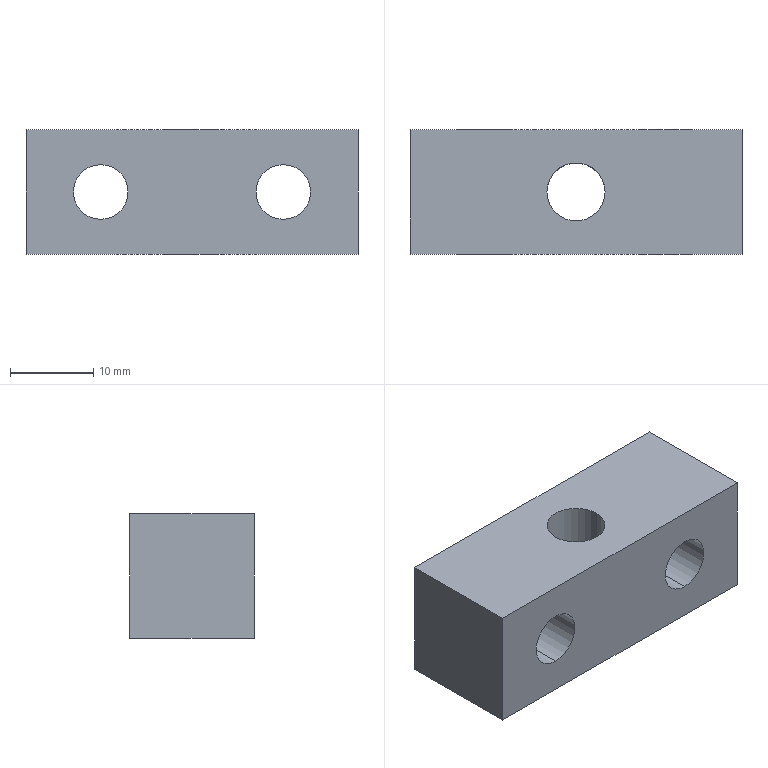Part | STEP file | 0243_212_Block | 1 solid | 12 faces | box 40 x 15 x 15 mm | volume 7396 mm3 | cylinder 6 | plane 6 | commonest cylinder face diameters 6.6 x4 7 x2
STEP:
#1=CARTESIAN_POINT('',(0.,0.,0.));
#2=DIRECTION('',(0.,0.,1.));
#3=DIRECTION('',(1.,0.,0.));
#4=AXIS2_PLACEMENT_3D('',#1,#2,#3);
#5=CARTESIAN_POINT('',(11.,0.,10.8));
#6=VERTEX_POINT('',#5);
#7=CARTESIAN_POINT('',(11.,15.,10.8));
#8=VERTEX_POINT('',#7);
#9=CARTESIAN_POINT('',(11.,15.,10.8));
#10=DIRECTION('',(0.,1.,0.));
#11=VECTOR('',#10,1.);
#12=LINE('',#9,#11);
#13=CARTESIAN_POINT('',(11.,15.,7.5));
#14=DIRECTION('',(0.,1.,0.));
#15=DIRECTION('',(0.,0.,1.));
#16=AXIS2_PLACEMENT_3D('',#13,#14,#15);
#17=CYLINDRICAL_SURFACE('',#16,3.3);
#18=CARTESIAN_POINT('',(6.283,0.));
#19=DIRECTION('',(0.,1.));
#20=VECTOR('',#19,1.);
#21=LINE('',#18,#20);
#22=(GEOMETRIC_REPRESENTATION_CONTEXT(2)PARAMETRIC_REPRESENTATION_CONTEXT()REPRESENTATION_CONTEXT('',''));
#23=DEFINITIONAL_REPRESENTATION('',(#21),#22);
#24=PCURVE('',#17,#23);
#25=CARTESIAN_POINT('',(11.,15.,7.5));
#26=DIRECTION('',(0.,1.,0.));
#27=DIRECTION('',(0.,0.,1.));
#28=AXIS2_PLACEMENT_3D('',#25,#26,#27);
#29=CYLINDRICAL_SURFACE('',#28,3.3);
#30=CARTESIAN_POINT('',(0.,0.));
#31=DIRECTION('',(0.,1.));
#32=VECTOR('',#31,1.);
#33=LINE('',#30,#32);
#34=(GEOMETRIC_REPRESENTATION_CONTEXT(2)PARAMETRIC_REPRESENTATION_CONTEXT()REPRESENTATION_CONTEXT('',''));
#35=DEFINITIONAL_REPRESENTATION('',(#33),#34);
#36=PCURVE('',#29,#35);
#37=SURFACE_CURVE('',#12,(#24,#36),.PCURVE_S1.);
#38=EDGE_CURVE('',#6,#8,#37,.T.);
#39=ORIENTED_EDGE('',*,*,#38,.T.);
#40=CARTESIAN_POINT('',(11.,15.,4.2));
#41=VERTEX_POINT('',#40);
#42=CARTESIAN_POINT('',(11.,15.,7.5));
#43=DIRECTION('',(0.,1.,0.));
#44=DIRECTION('',(0.,0.,1.));
#45=AXIS2_PLACEMENT_3D('',#42,#43,#44);
#46=CIRCLE('',#45,3.3);
#47=CARTESIAN_POINT('',(0.,0.));
#48=DIRECTION('',(1.,0.));
#49=VECTOR('',#48,1.);
#50=LINE('',#47,#49);
#51=(GEOMETRIC_REPRESENTATION_CONTEXT(2)PARAMETRIC_REPRESENTATION_CONTEXT()REPRESENTATION_CONTEXT('',''));
#52=DEFINITIONAL_REPRESENTATION('',(#50),#51);
#53=PCURVE('',#17,#52);
#54=CARTESIAN_POINT('',(-20.,15.,15.));
#55=DIRECTION('',(0.,-1.,0.));
#56=DIRECTION('',(0.,0.,-1.));
#57=AXIS2_PLACEMENT_3D('',#54,#55,#56);
#58=PLANE('',#57);
#59=CARTESIAN_POINT('',(4.2,31.));
#60=CARTESIAN_POINT('',(4.2,36.716));
#61=CARTESIAN_POINT('',(9.15,33.858));
#62=CARTESIAN_POINT('',(14.1,31.));
#63=CARTESIAN_POINT('',(9.15,28.142));
#64=CARTESIAN_POINT('',(4.2,25.284));
#65=CARTESIAN_POINT('',(4.2,31.));
#66=(BOUNDED_CURVE()B_SPLINE_CURVE(2,(#59,#60,#61,#62,#63,#64,#65),.UNSPECIFIED.,.T.,.F.)B_SPLINE_CURVE_WITH_KNOTS((1,2,2,2,2,1),(-2.094,0.,2.094,4.189,6.283,8.378),.UNSPECIFIED.)CURVE()GEOMETRIC_REPRESENTATION_ITEM()RATIONAL_B_SPLINE_CURVE((1.,0.5,1.,0.5,1.,0.5,1.))REPRESENTATION_ITEM(''));
#67=(GEOMETRIC_REPRESENTATION_CONTEXT(2)PARAMETRIC_REPRESENTATION_CONTEXT()REPRESENTATION_CONTEXT('',''));
#68=DEFINITIONAL_REPRESENTATION('',(#66),#67);
#69=PCURVE('',#58,#68);
#70=SURFACE_CURVE('',#46,(#53,#69),.PCURVE_S1.);
#71=EDGE_CURVE('',#41,#8,#70,.T.);
#72=ORIENTED_EDGE('',*,*,#71,.F.);
#73=CARTESIAN_POINT('',(11.,0.,4.2));
#74=VERTEX_POINT('',#73);
#75=CARTESIAN_POINT('',(11.,15.,4.2));
#76=DIRECTION('',(0.,1.,0.));
#77=VECTOR('',#76,1.);
#78=LINE('',#75,#77);
#79=CARTESIAN_POINT('',(3.142,0.));
#80=DIRECTION('',(0.,1.));
#81=VECTOR('',#80,1.);
#82=LINE('',#79,#81);
#83=(GEOMETRIC_REPRESENTATION_CONTEXT(2)PARAMETRIC_REPRESENTATION_CONTEXT()REPRESENTATION_CONTEXT('',''));
#84=DEFINITIONAL_REPRESENTATION('',(#82),#83);
#85=PCURVE('',#17,#84);
#86=CARTESIAN_POINT('',(3.142,0.));
#87=DIRECTION('',(0.,1.));
#88=VECTOR('',#87,1.);
#89=LINE('',#86,#88);
#90=(GEOMETRIC_REPRESENTATION_CONTEXT(2)PARAMETRIC_REPRESENTATION_CONTEXT()REPRESENTATION_CONTEXT('',''));
#91=DEFINITIONAL_REPRESENTATION('',(#89),#90);
#92=PCURVE('',#29,#91);
#93=SURFACE_CURVE('',#78,(#85,#92),.PCURVE_S1.);
#94=EDGE_CURVE('',#74,#41,#93,.T.);
#95=ORIENTED_EDGE('',*,*,#94,.F.);
#96=CARTESIAN_POINT('',(11.,0.,7.5));
#97=DIRECTION('',(0.,1.,0.));
#98=DIRECTION('',(0.,0.,1.));
#99=AXIS2_PLACEMENT_3D('',#96,#97,#98);
#100=CIRCLE('',#99,3.3);
#101=CARTESIAN_POINT('',(0.,-15.));
#102=DIRECTION('',(1.,0.));
#103=VECTOR('',#102,1.);
#104=LINE('',#101,#103);
#105=(GEOMETRIC_REPRESENTATION_CONTEXT(2)PARAMETRIC_REPRESENTATION_CONTEXT()REPRESENTATION_CONTEXT('',''));
#106=DEFINITIONAL_REPRESENTATION('',(#104),#105);
#107=PCURVE('',#17,#106);
#108=CARTESIAN_POINT('',(-20.,0.,15.));
#109=DIRECTION('',(0.,1.,0.));
#110=DIRECTION('',(0.,0.,1.));
#111=AXIS2_PLACEMENT_3D('',#108,#109,#110);
#112=PLANE('',#111);
#113=CARTESIAN_POINT('',(-7.5,31.));
#114=DIRECTION('',(1.,0.));
#115=AXIS2_PLACEMENT_2D('',#113,#114);
#116=CIRCLE('',#115,3.3);
#117=(GEOMETRIC_REPRESENTATION_CONTEXT(2)PARAMETRIC_REPRESENTATION_CONTEXT()REPRESENTATION_CONTEXT('',''));
#118=DEFINITIONAL_REPRESENTATION('',(#116),#117);
#119=PCURVE('',#112,#118);
#120=SURFACE_CURVE('',#100,(#107,#119),.PCURVE_S1.);
#121=EDGE_CURVE('',#74,#6,#120,.T.);
#122=ORIENTED_EDGE('',*,*,#121,.T.);
#123=EDGE_LOOP('',(#39,#72,#95,#122));
#124=FACE_BOUND('',#123,.F.);
#125=ADVANCED_FACE('',(#124),#17,.F.);
#126=CARTESIAN_POINT('',(-11.,0.,10.8));
#127=VERTEX_POINT('',#126);
#128=CARTESIAN_POINT('',(-11.,15.,10.8));
#129=VERTEX_POINT('',#128);
#130=CARTESIAN_POINT('',(-11.,15.,10.8));
#131=DIRECTION('',(0.,1.,0.));
#132=VECTOR('',#131,1.);
#133=LINE('',#130,#132);
#134=CARTESIAN_POINT('',(-11.,15.,7.5));
#135=DIRECTION('',(0.,1.,0.));
#136=DIRECTION('',(0.,0.,1.));
#137=AXIS2_PLACEMENT_3D('',#134,#135,#136);
#138=CYLINDRICAL_SURFACE('',#137,3.3);
#139=CARTESIAN_POINT('',(6.283,0.));
#140=DIRECTION('',(0.,1.));
#141=VECTOR('',#140,1.);
#142=LINE('',#139,#141);
#143=(GEOMETRIC_REPRESENTATION_CONTEXT(2)PARAMETRIC_REPRESENTATION_CONTEXT()REPRESENTATION_CONTEXT('',''));
#144=DEFINITIONAL_REPRESENTATION('',(#142),#143);
#145=PCURVE('',#138,#144);
#146=CARTESIAN_POINT('',(-11.,15.,7.5));
#147=DIRECTION('',(0.,1.,0.));
#148=DIRECTION('',(0.,0.,1.));
#149=AXIS2_PLACEMENT_3D('',#146,#147,#148);
#150=CYLINDRICAL_SURFACE('',#149,3.3);
#151=CARTESIAN_POINT('',(0.,0.));
#152=DIRECTION('',(0.,1.));
#153=VECTOR('',#152,1.);
#154=LINE('',#151,#153);
#155=(GEOMETRIC_REPRESENTATION_CONTEXT(2)PARAMETRIC_REPRESENTATION_CONTEXT()REPRESENTATION_CONTEXT('',''));
#156=DEFINITIONAL_REPRESENTATION('',(#154),#155);
#157=PCURVE('',#150,#156);
#158=SURFACE_CURVE('',#133,(#145,#157),.PCURVE_S1.);
#159=EDGE_CURVE('',#127,#129,#158,.T.);
#160=ORIENTED_EDGE('',*,*,#159,.T.);
#161=CARTESIAN_POINT('',(-11.,15.,4.2));
#162=VERTEX_POINT('',#161);
#163=CARTESIAN_POINT('',(-11.,15.,7.5));
#164=DIRECTION('',(0.,1.,0.));
#165=DIRECTION('',(0.,0.,1.));
#166=AXIS2_PLACEMENT_3D('',#163,#164,#165);
#167=CIRCLE('',#166,3.3);
#168=CARTESIAN_POINT('',(0.,0.));
#169=DIRECTION('',(1.,0.));
#170=VECTOR('',#169,1.);
#171=LINE('',#168,#170);
#172=(GEOMETRIC_REPRESENTATION_CONTEXT(2)PARAMETRIC_REPRESENTATION_CONTEXT()REPRESENTATION_CONTEXT('',''));
#173=DEFINITIONAL_REPRESENTATION('',(#171),#172);
#174=PCURVE('',#138,#173);
#175=CARTESIAN_POINT('',(4.2,9.));
#176=CARTESIAN_POINT('',(4.2,14.716));
#177=CARTESIAN_POINT('',(9.15,11.858));
#178=CARTESIAN_POINT('',(14.1,9.));
#179=CARTESIAN_POINT('',(9.15,6.142));
#180=CARTESIAN_POINT('',(4.2,3.284));
#181=CARTESIAN_POINT('',(4.2,9.));
#182=(BOUNDED_CURVE()B_SPLINE_CURVE(2,(#175,#176,#177,#178,#179,#180,#181),.UNSPECIFIED.,.T.,.F.)B_SPLINE_CURVE_WITH_KNOTS((1,2,2,2,2,1),(-2.094,0.,2.094,4.189,6.283,8.378),.UNSPECIFIED.)CURVE()GEOMETRIC_REPRESENTATION_ITEM()RATIONAL_B_SPLINE_CURVE((1.,0.5,1.,0.5,1.,0.5,1.))REPRESENTATION_ITEM(''));
#183=(GEOMETRIC_REPRESENTATION_CONTEXT(2)PARAMETRIC_REPRESENTATION_CONTEXT()REPRESENTATION_CONTEXT('',''));
#184=DEFINITIONAL_REPRESENTATION('',(#182),#183);
#185=PCURVE('',#58,#184);
#186=SURFACE_CURVE('',#167,(#174,#185),.PCURVE_S1.);
#187=EDGE_CURVE('',#162,#129,#186,.T.);
#188=ORIENTED_EDGE('',*,*,#187,.F.);
#189=CARTESIAN_POINT('',(-11.,0.,4.2));
#190=VERTEX_POINT('',#189);
#191=CARTESIAN_POINT('',(-11.,15.,4.2));
#192=DIRECTION('',(0.,1.,0.));
#193=VECTOR('',#192,1.);
#194=LINE('',#191,#193);
#195=CARTESIAN_POINT('',(3.142,0.));
#196=DIRECTION('',(0.,1.));
#197=VECTOR('',#196,1.);
#198=LINE('',#195,#197);
#199=(GEOMETRIC_REPRESENTATION_CONTEXT(2)PARAMETRIC_REPRESENTATION_CONTEXT()REPRESENTATION_CONTEXT('',''));
#200=DEFINITIONAL_REPRESENTATION('',(#198),#199);
#201=PCURVE('',#138,#200);
#202=CARTESIAN_POINT('',(3.142,0.));
#203=DIRECTION('',(0.,1.));
#204=VECTOR('',#203,1.);
#205=LINE('',#202,#204);
#206=(GEOMETRIC_REPRESENTATION_CONTEXT(2)PARAMETRIC_REPRESENTATION_CONTEXT()REPRESENTATION_CONTEXT('',''));
#207=DEFINITIONAL_REPRESENTATION('',(#205),#206);
#208=PCURVE('',#150,#207);
#209=SURFACE_CURVE('',#194,(#201,#208),.PCURVE_S1.);
#210=EDGE_CURVE('',#190,#162,#209,.T.);
#211=ORIENTED_EDGE('',*,*,#210,.F.);
#212=CARTESIAN_POINT('',(-11.,0.,7.5));
#213=DIRECTION('',(0.,1.,0.));
#214=DIRECTION('',(0.,0.,1.));
#215=AXIS2_PLACEMENT_3D('',#212,#213,#214);
#216=CIRCLE('',#215,3.3);
#217=CARTESIAN_POINT('',(0.,-15.));
#218=DIRECTION('',(1.,0.));
#219=VECTOR('',#218,1.);
#220=LINE('',#217,#219);
#221=(GEOMETRIC_REPRESENTATION_CONTEXT(2)PARAMETRIC_REPRESENTATION_CONTEXT()REPRESENTATION_CONTEXT('',''));
#222=DEFINITIONAL_REPRESENTATION('',(#220),#221);
#223=PCURVE('',#138,#222);
#224=CARTESIAN_POINT('',(-7.5,9.));
#225=DIRECTION('',(1.,0.));
#226=AXIS2_PLACEMENT_2D('',#224,#225);
#227=CIRCLE('',#226,3.3);
#228=(GEOMETRIC_REPRESENTATION_CONTEXT(2)PARAMETRIC_REPRESENTATION_CONTEXT()REPRESENTATION_CONTEXT('',''));
#229=DEFINITIONAL_REPRESENTATION('',(#227),#228);
#230=PCURVE('',#112,#229);
#231=SURFACE_CURVE('',#216,(#223,#230),.PCURVE_S1.);
#232=EDGE_CURVE('',#190,#127,#231,.T.);
#233=ORIENTED_EDGE('',*,*,#232,.T.);
#234=EDGE_LOOP('',(#160,#188,#211,#233));
#235=FACE_BOUND('',#234,.F.);
#236=ADVANCED_FACE('',(#235),#138,.F.);
#237=CARTESIAN_POINT('',(3.5,7.5,0.));
#238=VERTEX_POINT('',#237);
#239=CARTESIAN_POINT('',(3.5,7.5,15.));
#240=VERTEX_POINT('',#239);
#241=CARTESIAN_POINT('',(3.5,7.5,15.));
#242=DIRECTION('',(0.,0.,1.));
#243=VECTOR('',#242,1.);
#244=LINE('',#241,#243);
#245=CARTESIAN_POINT('',(0.,7.5,15.));
#246=DIRECTION('',(0.,0.,1.));
#247=DIRECTION('',(1.,0.,0.));
#248=AXIS2_PLACEMENT_3D('',#245,#246,#247);
#249=CYLINDRICAL_SURFACE('',#248,3.5);
#250=CARTESIAN_POINT('',(6.283,0.));
#251=DIRECTION('',(0.,1.));
#252=VECTOR('',#251,1.);
#253=LINE('',#250,#252);
#254=(GEOMETRIC_REPRESENTATION_CONTEXT(2)PARAMETRIC_REPRESENTATION_CONTEXT()REPRESENTATION_CONTEXT('',''));
#255=DEFINITIONAL_REPRESENTATION('',(#253),#254);
#256=PCURVE('',#249,#255);
#257=CARTESIAN_POINT('',(0.,7.5,15.));
#258=DIRECTION('',(0.,0.,1.));
#259=DIRECTION('',(1.,0.,0.));
#260=AXIS2_PLACEMENT_3D('',#257,#258,#259);
#261=CYLINDRICAL_SURFACE('',#260,3.5);
#262=CARTESIAN_POINT('',(0.,0.));
#263=DIRECTION('',(0.,1.));
#264=VECTOR('',#263,1.);
#265=LINE('',#262,#264);
#266=(GEOMETRIC_REPRESENTATION_CONTEXT(2)PARAMETRIC_REPRESENTATION_CONTEXT()REPRESENTATION_CONTEXT('',''));
#267=DEFINITIONAL_REPRESENTATION('',(#265),#266);
#268=PCURVE('',#261,#267);
#269=SURFACE_CURVE('',#244,(#256,#268),.PCURVE_S1.);
#270=EDGE_CURVE('',#238,#240,#269,.T.);
#271=ORIENTED_EDGE('',*,*,#270,.T.);
#272=CARTESIAN_POINT('',(-3.5,7.5,15.));
#273=VERTEX_POINT('',#272);
#274=CARTESIAN_POINT('',(0.,7.5,15.));
#275=DIRECTION('',(0.,0.,1.));
#276=DIRECTION('',(1.,0.,0.));
#277=AXIS2_PLACEMENT_3D('',#274,#275,#276);
#278=CIRCLE('',#277,3.5);
#279=CARTESIAN_POINT('',(0.,0.));
#280=DIRECTION('',(1.,0.));
#281=VECTOR('',#280,1.);
#282=LINE('',#279,#281);
#283=(GEOMETRIC_REPRESENTATION_CONTEXT(2)PARAMETRIC_REPRESENTATION_CONTEXT()REPRESENTATION_CONTEXT('',''));
#284=DEFINITIONAL_REPRESENTATION('',(#282),#283);
#285=PCURVE('',#249,#284);
#286=CARTESIAN_POINT('',(-20.,15.,15.));
#287=DIRECTION('',(0.,0.,-1.));
#288=DIRECTION('',(-1.,0.,0.));
#289=AXIS2_PLACEMENT_3D('',#286,#287,#288);
#290=PLANE('',#289);
#291=CARTESIAN_POINT('',(-23.5,-7.5));
#292=CARTESIAN_POINT('',(-23.5,-1.438));
#293=CARTESIAN_POINT('',(-18.25,-4.469));
#294=CARTESIAN_POINT('',(-13.,-7.5));
#295=CARTESIAN_POINT('',(-18.25,-10.531));
#296=CARTESIAN_POINT('',(-23.5,-13.562));
#297=CARTESIAN_POINT('',(-23.5,-7.5));
#298=(BOUNDED_CURVE()B_SPLINE_CURVE(2,(#291,#292,#293,#294,#295,#296,#297),.UNSPECIFIED.,.T.,.F.)B_SPLINE_CURVE_WITH_KNOTS((1,2,2,2,2,1),(-2.094,0.,2.094,4.189,6.283,8.378),.UNSPECIFIED.)CURVE()GEOMETRIC_REPRESENTATION_ITEM()RATIONAL_B_SPLINE_CURVE((1.,0.5,1.,0.5,1.,0.5,1.))REPRESENTATION_ITEM(''));
#299=(GEOMETRIC_REPRESENTATION_CONTEXT(2)PARAMETRIC_REPRESENTATION_CONTEXT()REPRESENTATION_CONTEXT('',''));
#300=DEFINITIONAL_REPRESENTATION('',(#298),#299);
#301=PCURVE('',#290,#300);
#302=SURFACE_CURVE('',#278,(#285,#301),.PCURVE_S1.);
#303=EDGE_CURVE('',#273,#240,#302,.T.);
#304=ORIENTED_EDGE('',*,*,#303,.F.);
#305=CARTESIAN_POINT('',(-3.5,7.5,0.));
#306=VERTEX_POINT('',#305);
#307=CARTESIAN_POINT('',(-3.5,7.5,15.));
#308=DIRECTION('',(0.,0.,1.));
#309=VECTOR('',#308,1.);
#310=LINE('',#307,#309);
#311=CARTESIAN_POINT('',(3.142,0.));
#312=DIRECTION('',(0.,1.));
#313=VECTOR('',#312,1.);
#314=LINE('',#311,#313);
#315=(GEOMETRIC_REPRESENTATION_CONTEXT(2)PARAMETRIC_REPRESENTATION_CONTEXT()REPRESENTATION_CONTEXT('',''));
#316=DEFINITIONAL_REPRESENTATION('',(#314),#315);
#317=PCURVE('',#249,#316);
#318=CARTESIAN_POINT('',(3.142,0.));
#319=DIRECTION('',(0.,1.));
#320=VECTOR('',#319,1.);
#321=LINE('',#318,#320);
#322=(GEOMETRIC_REPRESENTATION_CONTEXT(2)PARAMETRIC_REPRESENTATION_CONTEXT()REPRESENTATION_CONTEXT('',''));
#323=DEFINITIONAL_REPRESENTATION('',(#321),#322);
#324=PCURVE('',#261,#323);
#325=SURFACE_CURVE('',#310,(#317,#324),.PCURVE_S1.);
#326=EDGE_CURVE('',#306,#273,#325,.T.);
#327=ORIENTED_EDGE('',*,*,#326,.F.);
#328=CARTESIAN_POINT('',(0.,7.5,0.));
#329=DIRECTION('',(0.,0.,1.));
#330=DIRECTION('',(1.,0.,0.));
#331=AXIS2_PLACEMENT_3D('',#328,#329,#330);
#332=CIRCLE('',#331,3.5);
#333=CARTESIAN_POINT('',(0.,-15.));
#334=DIRECTION('',(1.,0.));
#335=VECTOR('',#334,1.);
#336=LINE('',#333,#335);
#337=(GEOMETRIC_REPRESENTATION_CONTEXT(2)PARAMETRIC_REPRESENTATION_CONTEXT()REPRESENTATION_CONTEXT('',''));
#338=DEFINITIONAL_REPRESENTATION('',(#336),#337);
#339=PCURVE('',#249,#338);
#340=CARTESIAN_POINT('',(-20.,15.,0.));
#341=DIRECTION('',(0.,0.,-1.));
#342=DIRECTION('',(-1.,0.,0.));
#343=AXIS2_PLACEMENT_3D('',#340,#341,#342);
#344=PLANE('',#343);
#345=CARTESIAN_POINT('',(-23.5,-7.5));
#346=CARTESIAN_POINT('',(-23.5,-1.438));
#347=CARTESIAN_POINT('',(-18.25,-4.469));
#348=CARTESIAN_POINT('',(-13.,-7.5));
#349=CARTESIAN_POINT('',(-18.25,-10.531));
#350=CARTESIAN_POINT('',(-23.5,-13.562));
#351=CARTESIAN_POINT('',(-23.5,-7.5));
#352=(BOUNDED_CURVE()B_SPLINE_CURVE(2,(#345,#346,#347,#348,#349,#350,#351),.UNSPECIFIED.,.T.,.F.)B_SPLINE_CURVE_WITH_KNOTS((1,2,2,2,2,1),(-2.094,0.,2.094,4.189,6.283,8.378),.UNSPECIFIED.)CURVE()GEOMETRIC_REPRESENTATION_ITEM()RATIONAL_B_SPLINE_CURVE((1.,0.5,1.,0.5,1.,0.5,1.))REPRESENTATION_ITEM(''));
#353=(GEOMETRIC_REPRESENTATION_CONTEXT(2)PARAMETRIC_REPRESENTATION_CONTEXT()REPRESENTATION_CONTEXT('',''));
#354=DEFINITIONAL_REPRESENTATION('',(#352),#353);
#355=PCURVE('',#344,#354);
#356=SURFACE_CURVE('',#332,(#339,#355),.PCURVE_S1.);
#357=EDGE_CURVE('',#306,#238,#356,.T.);
#358=ORIENTED_EDGE('',*,*,#357,.T.);
#359=EDGE_LOOP('',(#271,#304,#327,#358));
#360=FACE_BOUND('',#359,.F.);
#361=ADVANCED_FACE('',(#360),#249,.F.);
#362=CARTESIAN_POINT('',(-20.,15.,0.));
#363=VERTEX_POINT('',#362);
#364=CARTESIAN_POINT('',(-20.,0.,0.));
#365=VERTEX_POINT('',#364);
#366=CARTESIAN_POINT('',(-20.,0.,0.));
#367=DIRECTION('',(0.,-1.,0.));
#368=VECTOR('',#367,1.);
#369=LINE('',#366,#368);
#370=CARTESIAN_POINT('',(-20.,0.,15.));
#371=DIRECTION('',(1.,0.,0.));
#372=DIRECTION('',(0.,0.,-1.));
#373=AXIS2_PLACEMENT_3D('',#370,#371,#372);
#374=PLANE('',#373);
#375=CARTESIAN_POINT('',(15.,0.));
#376=DIRECTION('',(0.,-1.));
#377=VECTOR('',#376,1.);
#378=LINE('',#375,#377);
#379=(GEOMETRIC_REPRESENTATION_CONTEXT(2)PARAMETRIC_REPRESENTATION_CONTEXT()REPRESENTATION_CONTEXT('',''));
#380=DEFINITIONAL_REPRESENTATION('',(#378),#379);
#381=PCURVE('',#374,#380);
#382=CARTESIAN_POINT('',(0.,-15.));
#383=DIRECTION('',(0.,-1.));
#384=VECTOR('',#383,1.);
#385=LINE('',#382,#384);
#386=(GEOMETRIC_REPRESENTATION_CONTEXT(2)PARAMETRIC_REPRESENTATION_CONTEXT()REPRESENTATION_CONTEXT('',''));
#387=DEFINITIONAL_REPRESENTATION('',(#385),#386);
#388=PCURVE('',#344,#387);
#389=SURFACE_CURVE('',#369,(#381,#388),.PCURVE_S1.);
#390=EDGE_CURVE('',#363,#365,#389,.T.);
#391=ORIENTED_EDGE('',*,*,#390,.T.);
#392=CARTESIAN_POINT('',(-20.,0.,15.));
#393=VERTEX_POINT('',#392);
#394=CARTESIAN_POINT('',(-20.,0.,15.));
#395=DIRECTION('',(0.,0.,-1.));
#396=VECTOR('',#395,1.);
#397=LINE('',#394,#396);
#398=CARTESIAN_POINT('',(0.,0.));
#399=DIRECTION('',(1.,0.));
#400=VECTOR('',#399,1.);
#401=LINE('',#398,#400);
#402=(GEOMETRIC_REPRESENTATION_CONTEXT(2)PARAMETRIC_REPRESENTATION_CONTEXT()REPRESENTATION_CONTEXT('',''));
#403=DEFINITIONAL_REPRESENTATION('',(#401),#402);
#404=PCURVE('',#374,#403);
#405=CARTESIAN_POINT('',(0.,0.));
#406=DIRECTION('',(-1.,0.));
#407=VECTOR('',#406,1.);
#408=LINE('',#405,#407);
#409=(GEOMETRIC_REPRESENTATION_CONTEXT(2)PARAMETRIC_REPRESENTATION_CONTEXT()REPRESENTATION_CONTEXT('',''));
#410=DEFINITIONAL_REPRESENTATION('',(#408),#409);
#411=PCURVE('',#112,#410);
#412=SURFACE_CURVE('',#397,(#404,#411),.PCURVE_S1.);
#413=EDGE_CURVE('',#393,#365,#412,.T.);
#414=ORIENTED_EDGE('',*,*,#413,.F.);
#415=CARTESIAN_POINT('',(-20.,15.,15.));
#416=VERTEX_POINT('',#415);
#417=CARTESIAN_POINT('',(-20.,0.,15.));
#418=DIRECTION('',(0.,-1.,0.));
#419=VECTOR('',#418,1.);
#420=LINE('',#417,#419);
#421=CARTESIAN_POINT('',(0.,0.));
#422=DIRECTION('',(0.,-1.));
#423=VECTOR('',#422,1.);
#424=LINE('',#421,#423);
#425=(GEOMETRIC_REPRESENTATION_CONTEXT(2)PARAMETRIC_REPRESENTATION_CONTEXT()REPRESENTATION_CONTEXT('',''));
#426=DEFINITIONAL_REPRESENTATION('',(#424),#425);
#427=PCURVE('',#374,#426);
#428=CARTESIAN_POINT('',(0.,-15.));
#429=DIRECTION('',(0.,-1.));
#430=VECTOR('',#429,1.);
#431=LINE('',#428,#430);
#432=(GEOMETRIC_REPRESENTATION_CONTEXT(2)PARAMETRIC_REPRESENTATION_CONTEXT()REPRESENTATION_CONTEXT('',''));
#433=DEFINITIONAL_REPRESENTATION('',(#431),#432);
#434=PCURVE('',#290,#433);
#435=SURFACE_CURVE('',#420,(#427,#434),.PCURVE_S1.);
#436=EDGE_CURVE('',#416,#393,#435,.T.);
#437=ORIENTED_EDGE('',*,*,#436,.F.);
#438=CARTESIAN_POINT('',(-20.,15.,15.));
#439=DIRECTION('',(0.,0.,-1.));
#440=VECTOR('',#439,1.);
#441=LINE('',#438,#440);
#442=CARTESIAN_POINT('',(0.,15.));
#443=DIRECTION('',(1.,0.));
#444=VECTOR('',#443,1.);
#445=LINE('',#442,#444);
#446=(GEOMETRIC_REPRESENTATION_CONTEXT(2)PARAMETRIC_REPRESENTATION_CONTEXT()REPRESENTATION_CONTEXT('',''));
#447=DEFINITIONAL_REPRESENTATION('',(#445),#446);
#448=PCURVE('',#374,#447);
#449=CARTESIAN_POINT('',(0.,0.));
#450=DIRECTION('',(1.,0.));
#451=VECTOR('',#450,1.);
#452=LINE('',#449,#451);
#453=(GEOMETRIC_REPRESENTATION_CONTEXT(2)PARAMETRIC_REPRESENTATION_CONTEXT()REPRESENTATION_CONTEXT('',''));
#454=DEFINITIONAL_REPRESENTATION('',(#452),#453);
#455=PCURVE('',#58,#454);
#456=SURFACE_CURVE('',#441,(#448,#455),.PCURVE_S1.);
#457=EDGE_CURVE('',#416,#363,#456,.T.);
#458=ORIENTED_EDGE('',*,*,#457,.T.);
#459=EDGE_LOOP('',(#391,#414,#437,#458));
#460=FACE_BOUND('',#459,.T.);
#461=ADVANCED_FACE('',(#460),#374,.F.);
#462=CARTESIAN_POINT('',(11.,0.,7.5));
#463=DIRECTION('',(0.,1.,0.));
#464=DIRECTION('',(0.,0.,1.));
#465=AXIS2_PLACEMENT_3D('',#462,#463,#464);
#466=CIRCLE('',#465,3.3);
#467=CARTESIAN_POINT('',(-7.5,31.));
#468=DIRECTION('',(1.,0.));
#469=AXIS2_PLACEMENT_2D('',#467,#468);
#470=CIRCLE('',#469,3.3);
#471=(GEOMETRIC_REPRESENTATION_CONTEXT(2)PARAMETRIC_REPRESENTATION_CONTEXT()REPRESENTATION_CONTEXT('',''));
#472=DEFINITIONAL_REPRESENTATION('',(#470),#471);
#473=PCURVE('',#112,#472);
#474=CARTESIAN_POINT('',(0.,-15.));
#475=DIRECTION('',(1.,0.));
#476=VECTOR('',#475,1.);
#477=LINE('',#474,#476);
#478=(GEOMETRIC_REPRESENTATION_CONTEXT(2)PARAMETRIC_REPRESENTATION_CONTEXT()REPRESENTATION_CONTEXT('',''));
#479=DEFINITIONAL_REPRESENTATION('',(#477),#478);
#480=PCURVE('',#29,#479);
#481=SURFACE_CURVE('',#466,(#473,#480),.PCURVE_S1.);
#482=EDGE_CURVE('',#6,#74,#481,.T.);
#483=ORIENTED_EDGE('',*,*,#482,.T.);
#484=ORIENTED_EDGE('',*,*,#121,.T.);
#485=EDGE_LOOP('',(#483,#484));
#486=FACE_BOUND('',#485,.T.);
#487=CARTESIAN_POINT('',(-11.,0.,7.5));
#488=DIRECTION('',(0.,1.,0.));
#489=DIRECTION('',(0.,0.,1.));
#490=AXIS2_PLACEMENT_3D('',#487,#488,#489);
#491=CIRCLE('',#490,3.3);
#492=CARTESIAN_POINT('',(-7.5,9.));
#493=DIRECTION('',(1.,0.));
#494=AXIS2_PLACEMENT_2D('',#492,#493);
#495=CIRCLE('',#494,3.3);
#496=(GEOMETRIC_REPRESENTATION_CONTEXT(2)PARAMETRIC_REPRESENTATION_CONTEXT()REPRESENTATION_CONTEXT('',''));
#497=DEFINITIONAL_REPRESENTATION('',(#495),#496);
#498=PCURVE('',#112,#497);
#499=CARTESIAN_POINT('',(0.,-15.));
#500=DIRECTION('',(1.,0.));
#501=VECTOR('',#500,1.);
#502=LINE('',#499,#501);
#503=(GEOMETRIC_REPRESENTATION_CONTEXT(2)PARAMETRIC_REPRESENTATION_CONTEXT()REPRESENTATION_CONTEXT('',''));
#504=DEFINITIONAL_REPRESENTATION('',(#502),#503);
#505=PCURVE('',#150,#504);
#506=SURFACE_CURVE('',#491,(#498,#505),.PCURVE_S1.);
#507=EDGE_CURVE('',#127,#190,#506,.T.);
#508=ORIENTED_EDGE('',*,*,#507,.T.);
#509=ORIENTED_EDGE('',*,*,#232,.T.);
#510=EDGE_LOOP('',(#508,#509));
#511=FACE_BOUND('',#510,.T.);
#512=CARTESIAN_POINT('',(20.,0.,0.));
#513=VERTEX_POINT('',#512);
#514=CARTESIAN_POINT('',(-20.,0.,0.));
#515=DIRECTION('',(1.,0.,0.));
#516=VECTOR('',#515,1.);
#517=LINE('',#514,#516);
#518=CARTESIAN_POINT('',(-15.,0.));
#519=DIRECTION('',(0.,1.));
#520=VECTOR('',#519,1.);
#521=LINE('',#518,#520);
#522=(GEOMETRIC_REPRESENTATION_CONTEXT(2)PARAMETRIC_REPRESENTATION_CONTEXT()REPRESENTATION_CONTEXT('',''));
#523=DEFINITIONAL_REPRESENTATION('',(#521),#522);
#524=PCURVE('',#112,#523);
#525=CARTESIAN_POINT('',(0.,-15.));
#526=DIRECTION('',(-1.,0.));
#527=VECTOR('',#526,1.);
#528=LINE('',#525,#527);
#529=(GEOMETRIC_REPRESENTATION_CONTEXT(2)PARAMETRIC_REPRESENTATION_CONTEXT()REPRESENTATION_CONTEXT('',''));
#530=DEFINITIONAL_REPRESENTATION('',(#528),#529);
#531=PCURVE('',#344,#530);
#532=SURFACE_CURVE('',#517,(#524,#531),.PCURVE_S1.);
#533=EDGE_CURVE('',#365,#513,#532,.T.);
#534=ORIENTED_EDGE('',*,*,#533,.T.);
#535=CARTESIAN_POINT('',(20.,0.,15.));
#536=VERTEX_POINT('',#535);
#537=CARTESIAN_POINT('',(20.,0.,15.));
#538=DIRECTION('',(0.,0.,-1.));
#539=VECTOR('',#538,1.);
#540=LINE('',#537,#539);
#541=CARTESIAN_POINT('',(0.,40.));
#542=DIRECTION('',(-1.,0.));
#543=VECTOR('',#542,1.);
#544=LINE('',#541,#543);
#545=(GEOMETRIC_REPRESENTATION_CONTEXT(2)PARAMETRIC_REPRESENTATION_CONTEXT()REPRESENTATION_CONTEXT('',''));
#546=DEFINITIONAL_REPRESENTATION('',(#544),#545);
#547=PCURVE('',#112,#546);
#548=CARTESIAN_POINT('',(20.,0.,15.));
#549=DIRECTION('',(-1.,0.,0.));
#550=DIRECTION('',(0.,0.,1.));
#551=AXIS2_PLACEMENT_3D('',#548,#549,#550);
#552=PLANE('',#551);
#553=CARTESIAN_POINT('',(0.,0.));
#554=DIRECTION('',(-1.,0.));
#555=VECTOR('',#554,1.);
#556=LINE('',#553,#555);
#557=(GEOMETRIC_REPRESENTATION_CONTEXT(2)PARAMETRIC_REPRESENTATION_CONTEXT()REPRESENTATION_CONTEXT('',''));
#558=DEFINITIONAL_REPRESENTATION('',(#556),#557);
#559=PCURVE('',#552,#558);
#560=SURFACE_CURVE('',#540,(#547,#559),.PCURVE_S1.);
#561=EDGE_CURVE('',#536,#513,#560,.T.);
#562=ORIENTED_EDGE('',*,*,#561,.F.);
#563=CARTESIAN_POINT('',(-20.,0.,15.));
#564=DIRECTION('',(1.,0.,0.));
#565=VECTOR('',#564,1.);
#566=LINE('',#563,#565);
#567=CARTESIAN_POINT('',(0.,0.));
#568=DIRECTION('',(0.,1.));
#569=VECTOR('',#568,1.);
#570=LINE('',#567,#569);
#571=(GEOMETRIC_REPRESENTATION_CONTEXT(2)PARAMETRIC_REPRESENTATION_CONTEXT()REPRESENTATION_CONTEXT('',''));
#572=DEFINITIONAL_REPRESENTATION('',(#570),#571);
#573=PCURVE('',#112,#572);
#574=CARTESIAN_POINT('',(0.,-15.));
#575=DIRECTION('',(-1.,0.));
#576=VECTOR('',#575,1.);
#577=LINE('',#574,#576);
#578=(GEOMETRIC_REPRESENTATION_CONTEXT(2)PARAMETRIC_REPRESENTATION_CONTEXT()REPRESENTATION_CONTEXT('',''));
#579=DEFINITIONAL_REPRESENTATION('',(#577),#578);
#580=PCURVE('',#290,#579);
#581=SURFACE_CURVE('',#566,(#573,#580),.PCURVE_S1.);
#582=EDGE_CURVE('',#393,#536,#581,.T.);
#583=ORIENTED_EDGE('',*,*,#582,.F.);
#584=ORIENTED_EDGE('',*,*,#413,.T.);
#585=EDGE_LOOP('',(#534,#562,#583,#584));
#586=FACE_BOUND('',#585,.T.);
#587=ADVANCED_FACE('',(#486,#511,#586),#112,.F.);
#588=CARTESIAN_POINT('',(20.,15.,0.));
#589=VERTEX_POINT('',#588);
#590=CARTESIAN_POINT('',(20.,0.,0.));
#591=DIRECTION('',(0.,1.,0.));
#592=VECTOR('',#591,1.);
#593=LINE('',#590,#592);
#594=CARTESIAN_POINT('',(-15.,0.));
#595=DIRECTION('',(0.,1.));
#596=VECTOR('',#595,1.);
#597=LINE('',#594,#596);
#598=(GEOMETRIC_REPRESENTATION_CONTEXT(2)PARAMETRIC_REPRESENTATION_CONTEXT()REPRESENTATION_CONTEXT('',''));
#599=DEFINITIONAL_REPRESENTATION('',(#597),#598);
#600=PCURVE('',#552,#599);
#601=CARTESIAN_POINT('',(-40.,-15.));
#602=DIRECTION('',(0.,1.));
#603=VECTOR('',#602,1.);
#604=LINE('',#601,#603);
#605=(GEOMETRIC_REPRESENTATION_CONTEXT(2)PARAMETRIC_REPRESENTATION_CONTEXT()REPRESENTATION_CONTEXT('',''));
#606=DEFINITIONAL_REPRESENTATION('',(#604),#605);
#607=PCURVE('',#344,#606);
#608=SURFACE_CURVE('',#593,(#600,#607),.PCURVE_S1.);
#609=EDGE_CURVE('',#513,#589,#608,.T.);
#610=ORIENTED_EDGE('',*,*,#609,.T.);
#611=CARTESIAN_POINT('',(20.,15.,15.));
#612=VERTEX_POINT('',#611);
#613=CARTESIAN_POINT('',(20.,15.,15.));
#614=DIRECTION('',(0.,0.,-1.));
#615=VECTOR('',#614,1.);
#616=LINE('',#613,#615);
#617=CARTESIAN_POINT('',(0.,15.));
#618=DIRECTION('',(-1.,0.));
#619=VECTOR('',#618,1.);
#620=LINE('',#617,#619);
#621=(GEOMETRIC_REPRESENTATION_CONTEXT(2)PARAMETRIC_REPRESENTATION_CONTEXT()REPRESENTATION_CONTEXT('',''));
#622=DEFINITIONAL_REPRESENTATION('',(#620),#621);
#623=PCURVE('',#552,#622);
#624=CARTESIAN_POINT('',(0.,40.));
#625=DIRECTION('',(1.,0.));
#626=VECTOR('',#625,1.);
#627=LINE('',#624,#626);
#628=(GEOMETRIC_REPRESENTATION_CONTEXT(2)PARAMETRIC_REPRESENTATION_CONTEXT()REPRESENTATION_CONTEXT('',''));
#629=DEFINITIONAL_REPRESENTATION('',(#627),#628);
#630=PCURVE('',#58,#629);
#631=SURFACE_CURVE('',#616,(#623,#630),.PCURVE_S1.);
#632=EDGE_CURVE('',#612,#589,#631,.T.);
#633=ORIENTED_EDGE('',*,*,#632,.F.);
#634=CARTESIAN_POINT('',(20.,0.,15.));
#635=DIRECTION('',(0.,1.,0.));
#636=VECTOR('',#635,1.);
#637=LINE('',#634,#636);
#638=CARTESIAN_POINT('',(0.,0.));
#639=DIRECTION('',(0.,1.));
#640=VECTOR('',#639,1.);
#641=LINE('',#638,#640);
#642=(GEOMETRIC_REPRESENTATION_CONTEXT(2)PARAMETRIC_REPRESENTATION_CONTEXT()REPRESENTATION_CONTEXT('',''));
#643=DEFINITIONAL_REPRESENTATION('',(#641),#642);
#644=PCURVE('',#552,#643);
#645=CARTESIAN_POINT('',(-40.,-15.));
#646=DIRECTION('',(0.,1.));
#647=VECTOR('',#646,1.);
#648=LINE('',#645,#647);
#649=(GEOMETRIC_REPRESENTATION_CONTEXT(2)PARAMETRIC_REPRESENTATION_CONTEXT()REPRESENTATION_CONTEXT('',''));
#650=DEFINITIONAL_REPRESENTATION('',(#648),#649);
#651=PCURVE('',#290,#650);
#652=SURFACE_CURVE('',#637,(#644,#651),.PCURVE_S1.);
#653=EDGE_CURVE('',#536,#612,#652,.T.);
#654=ORIENTED_EDGE('',*,*,#653,.F.);
#655=ORIENTED_EDGE('',*,*,#561,.T.);
#656=EDGE_LOOP('',(#610,#633,#654,#655));
#657=FACE_BOUND('',#656,.T.);
#658=ADVANCED_FACE('',(#657),#552,.F.);
#659=CARTESIAN_POINT('',(11.,15.,7.5));
#660=DIRECTION('',(0.,1.,0.));
#661=DIRECTION('',(0.,0.,1.));
#662=AXIS2_PLACEMENT_3D('',#659,#660,#661);
#663=CIRCLE('',#662,3.3);
#664=CARTESIAN_POINT('',(4.2,31.));
#665=CARTESIAN_POINT('',(4.2,36.716));
#666=CARTESIAN_POINT('',(9.15,33.858));
#667=CARTESIAN_POINT('',(14.1,31.));
#668=CARTESIAN_POINT('',(9.15,28.142));
#669=CARTESIAN_POINT('',(4.2,25.284));
#670=CARTESIAN_POINT('',(4.2,31.));
#671=(BOUNDED_CURVE()B_SPLINE_CURVE(2,(#664,#665,#666,#667,#668,#669,#670),.UNSPECIFIED.,.T.,.F.)B_SPLINE_CURVE_WITH_KNOTS((1,2,2,2,2,1),(-2.094,0.,2.094,4.189,6.283,8.378),.UNSPECIFIED.)CURVE()GEOMETRIC_REPRESENTATION_ITEM()RATIONAL_B_SPLINE_CURVE((1.,0.5,1.,0.5,1.,0.5,1.))REPRESENTATION_ITEM(''));
#672=(GEOMETRIC_REPRESENTATION_CONTEXT(2)PARAMETRIC_REPRESENTATION_CONTEXT()REPRESENTATION_CONTEXT('',''));
#673=DEFINITIONAL_REPRESENTATION('',(#671),#672);
#674=PCURVE('',#58,#673);
#675=CARTESIAN_POINT('',(0.,0.));
#676=DIRECTION('',(1.,0.));
#677=VECTOR('',#676,1.);
#678=LINE('',#675,#677);
#679=(GEOMETRIC_REPRESENTATION_CONTEXT(2)PARAMETRIC_REPRESENTATION_CONTEXT()REPRESENTATION_CONTEXT('',''));
#680=DEFINITIONAL_REPRESENTATION('',(#678),#679);
#681=PCURVE('',#29,#680);
#682=SURFACE_CURVE('',#663,(#674,#681),.PCURVE_S1.);
#683=EDGE_CURVE('',#8,#41,#682,.T.);
#684=ORIENTED_EDGE('',*,*,#683,.F.);
#685=ORIENTED_EDGE('',*,*,#71,.F.);
#686=EDGE_LOOP('',(#684,#685));
#687=FACE_BOUND('',#686,.T.);
#688=CARTESIAN_POINT('',(-11.,15.,7.5));
#689=DIRECTION('',(0.,1.,0.));
#690=DIRECTION('',(0.,0.,1.));
#691=AXIS2_PLACEMENT_3D('',#688,#689,#690);
#692=CIRCLE('',#691,3.3);
#693=CARTESIAN_POINT('',(4.2,9.));
#694=CARTESIAN_POINT('',(4.2,14.716));
#695=CARTESIAN_POINT('',(9.15,11.858));
#696=CARTESIAN_POINT('',(14.1,9.));
#697=CARTESIAN_POINT('',(9.15,6.142));
#698=CARTESIAN_POINT('',(4.2,3.284));
#699=CARTESIAN_POINT('',(4.2,9.));
#700=(BOUNDED_CURVE()B_SPLINE_CURVE(2,(#693,#694,#695,#696,#697,#698,#699),.UNSPECIFIED.,.T.,.F.)B_SPLINE_CURVE_WITH_KNOTS((1,2,2,2,2,1),(-2.094,0.,2.094,4.189,6.283,8.378),.UNSPECIFIED.)CURVE()GEOMETRIC_REPRESENTATION_ITEM()RATIONAL_B_SPLINE_CURVE((1.,0.5,1.,0.5,1.,0.5,1.))REPRESENTATION_ITEM(''));
#701=(GEOMETRIC_REPRESENTATION_CONTEXT(2)PARAMETRIC_REPRESENTATION_CONTEXT()REPRESENTATION_CONTEXT('',''));
#702=DEFINITIONAL_REPRESENTATION('',(#700),#701);
#703=PCURVE('',#58,#702);
#704=CARTESIAN_POINT('',(0.,0.));
#705=DIRECTION('',(1.,0.));
#706=VECTOR('',#705,1.);
#707=LINE('',#704,#706);
#708=(GEOMETRIC_REPRESENTATION_CONTEXT(2)PARAMETRIC_REPRESENTATION_CONTEXT()REPRESENTATION_CONTEXT('',''));
#709=DEFINITIONAL_REPRESENTATION('',(#707),#708);
#710=PCURVE('',#150,#709);
#711=SURFACE_CURVE('',#692,(#703,#710),.PCURVE_S1.);
#712=EDGE_CURVE('',#129,#162,#711,.T.);
#713=ORIENTED_EDGE('',*,*,#712,.F.);
#714=ORIENTED_EDGE('',*,*,#187,.F.);
#715=EDGE_LOOP('',(#713,#714));
#716=FACE_BOUND('',#715,.T.);
#717=CARTESIAN_POINT('',(-20.,15.,0.));
#718=DIRECTION('',(-1.,0.,0.));
#719=VECTOR('',#718,1.);
#720=LINE('',#717,#719);
#721=CARTESIAN_POINT('',(15.,0.));
#722=DIRECTION('',(0.,-1.));
#723=VECTOR('',#722,1.);
#724=LINE('',#721,#723);
#725=(GEOMETRIC_REPRESENTATION_CONTEXT(2)PARAMETRIC_REPRESENTATION_CONTEXT()REPRESENTATION_CONTEXT('',''));
#726=DEFINITIONAL_REPRESENTATION('',(#724),#725);
#727=PCURVE('',#58,#726);
#728=CARTESIAN_POINT('',(0.,0.));
#729=DIRECTION('',(1.,0.));
#730=VECTOR('',#729,1.);
#731=LINE('',#728,#730);
#732=(GEOMETRIC_REPRESENTATION_CONTEXT(2)PARAMETRIC_REPRESENTATION_CONTEXT()REPRESENTATION_CONTEXT('',''));
#733=DEFINITIONAL_REPRESENTATION('',(#731),#732);
#734=PCURVE('',#344,#733);
#735=SURFACE_CURVE('',#720,(#727,#734),.PCURVE_S1.);
#736=EDGE_CURVE('',#589,#363,#735,.T.);
#737=ORIENTED_EDGE('',*,*,#736,.T.);
#738=ORIENTED_EDGE('',*,*,#457,.F.);
#739=CARTESIAN_POINT('',(-20.,15.,15.));
#740=DIRECTION('',(-1.,0.,0.));
#741=VECTOR('',#740,1.);
#742=LINE('',#739,#741);
#743=CARTESIAN_POINT('',(0.,0.));
#744=DIRECTION('',(0.,-1.));
#745=VECTOR('',#744,1.);
#746=LINE('',#743,#745);
#747=(GEOMETRIC_REPRESENTATION_CONTEXT(2)PARAMETRIC_REPRESENTATION_CONTEXT()REPRESENTATION_CONTEXT('',''));
#748=DEFINITIONAL_REPRESENTATION('',(#746),#747);
#749=PCURVE('',#58,#748);
#750=CARTESIAN_POINT('',(0.,0.));
#751=DIRECTION('',(1.,0.));
#752=VECTOR('',#751,1.);
#753=LINE('',#750,#752);
#754=(GEOMETRIC_REPRESENTATION_CONTEXT(2)PARAMETRIC_REPRESENTATION_CONTEXT()REPRESENTATION_CONTEXT('',''));
#755=DEFINITIONAL_REPRESENTATION('',(#753),#754);
#756=PCURVE('',#290,#755);
#757=SURFACE_CURVE('',#742,(#749,#756),.PCURVE_S1.);
#758=EDGE_CURVE('',#612,#416,#757,.T.);
#759=ORIENTED_EDGE('',*,*,#758,.F.);
#760=ORIENTED_EDGE('',*,*,#632,.T.);
#761=EDGE_LOOP('',(#737,#738,#759,#760));
#762=FACE_BOUND('',#761,.T.);
#763=ADVANCED_FACE('',(#687,#716,#762),#58,.F.);
#764=CARTESIAN_POINT('',(0.,7.5,15.));
#765=DIRECTION('',(0.,0.,1.));
#766=DIRECTION('',(1.,0.,0.));
#767=AXIS2_PLACEMENT_3D('',#764,#765,#766);
#768=CIRCLE('',#767,3.5);
#769=CARTESIAN_POINT('',(-23.5,-7.5));
#770=CARTESIAN_POINT('',(-23.5,-1.438));
#771=CARTESIAN_POINT('',(-18.25,-4.469));
#772=CARTESIAN_POINT('',(-13.,-7.5));
#773=CARTESIAN_POINT('',(-18.25,-10.531));
#774=CARTESIAN_POINT('',(-23.5,-13.562));
#775=CARTESIAN_POINT('',(-23.5,-7.5));
#776=(BOUNDED_CURVE()B_SPLINE_CURVE(2,(#769,#770,#771,#772,#773,#774,#775),.UNSPECIFIED.,.T.,.F.)B_SPLINE_CURVE_WITH_KNOTS((1,2,2,2,2,1),(-2.094,0.,2.094,4.189,6.283,8.378),.UNSPECIFIED.)CURVE()GEOMETRIC_REPRESENTATION_ITEM()RATIONAL_B_SPLINE_CURVE((1.,0.5,1.,0.5,1.,0.5,1.))REPRESENTATION_ITEM(''));
#777=(GEOMETRIC_REPRESENTATION_CONTEXT(2)PARAMETRIC_REPRESENTATION_CONTEXT()REPRESENTATION_CONTEXT('',''));
#778=DEFINITIONAL_REPRESENTATION('',(#776),#777);
#779=PCURVE('',#290,#778);
#780=CARTESIAN_POINT('',(0.,0.));
#781=DIRECTION('',(1.,0.));
#782=VECTOR('',#781,1.);
#783=LINE('',#780,#782);
#784=(GEOMETRIC_REPRESENTATION_CONTEXT(2)PARAMETRIC_REPRESENTATION_CONTEXT()REPRESENTATION_CONTEXT('',''));
#785=DEFINITIONAL_REPRESENTATION('',(#783),#784);
#786=PCURVE('',#261,#785);
#787=SURFACE_CURVE('',#768,(#779,#786),.PCURVE_S1.);
#788=EDGE_CURVE('',#240,#273,#787,.T.);
#789=ORIENTED_EDGE('',*,*,#788,.F.);
#790=ORIENTED_EDGE('',*,*,#303,.F.);
#791=EDGE_LOOP('',(#789,#790));
#792=FACE_BOUND('',#791,.T.);
#793=ORIENTED_EDGE('',*,*,#436,.T.);
#794=ORIENTED_EDGE('',*,*,#582,.T.);
#795=ORIENTED_EDGE('',*,*,#653,.T.);
#796=ORIENTED_EDGE('',*,*,#758,.T.);
#797=EDGE_LOOP('',(#793,#794,#795,#796));
#798=FACE_BOUND('',#797,.T.);
#799=ADVANCED_FACE('',(#792,#798),#290,.F.);
#800=CARTESIAN_POINT('',(0.,7.5,0.));
#801=DIRECTION('',(0.,0.,1.));
#802=DIRECTION('',(1.,0.,0.));
#803=AXIS2_PLACEMENT_3D('',#800,#801,#802);
#804=CIRCLE('',#803,3.5);
#805=CARTESIAN_POINT('',(-23.5,-7.5));
#806=CARTESIAN_POINT('',(-23.5,-1.438));
#807=CARTESIAN_POINT('',(-18.25,-4.469));
#808=CARTESIAN_POINT('',(-13.,-7.5));
#809=CARTESIAN_POINT('',(-18.25,-10.531));
#810=CARTESIAN_POINT('',(-23.5,-13.562));
#811=CARTESIAN_POINT('',(-23.5,-7.5));
#812=(BOUNDED_CURVE()B_SPLINE_CURVE(2,(#805,#806,#807,#808,#809,#810,#811),.UNSPECIFIED.,.T.,.F.)B_SPLINE_CURVE_WITH_KNOTS((1,2,2,2,2,1),(-2.094,0.,2.094,4.189,6.283,8.378),.UNSPECIFIED.)CURVE()GEOMETRIC_REPRESENTATION_ITEM()RATIONAL_B_SPLINE_CURVE((1.,0.5,1.,0.5,1.,0.5,1.))REPRESENTATION_ITEM(''));
#813=(GEOMETRIC_REPRESENTATION_CONTEXT(2)PARAMETRIC_REPRESENTATION_CONTEXT()REPRESENTATION_CONTEXT('',''));
#814=DEFINITIONAL_REPRESENTATION('',(#812),#813);
#815=PCURVE('',#344,#814);
#816=CARTESIAN_POINT('',(0.,-15.));
#817=DIRECTION('',(1.,0.));
#818=VECTOR('',#817,1.);
#819=LINE('',#816,#818);
#820=(GEOMETRIC_REPRESENTATION_CONTEXT(2)PARAMETRIC_REPRESENTATION_CONTEXT()REPRESENTATION_CONTEXT('',''));
#821=DEFINITIONAL_REPRESENTATION('',(#819),#820);
#822=PCURVE('',#261,#821);
#823=SURFACE_CURVE('',#804,(#815,#822),.PCURVE_S1.);
#824=EDGE_CURVE('',#238,#306,#823,.T.);
#825=ORIENTED_EDGE('',*,*,#824,.T.);
#826=ORIENTED_EDGE('',*,*,#357,.T.);
#827=EDGE_LOOP('',(#825,#826));
#828=FACE_BOUND('',#827,.T.);
#829=ORIENTED_EDGE('',*,*,#390,.F.);
#830=ORIENTED_EDGE('',*,*,#736,.F.);
#831=ORIENTED_EDGE('',*,*,#609,.F.);
#832=ORIENTED_EDGE('',*,*,#533,.F.);
#833=EDGE_LOOP('',(#829,#830,#831,#832));
#834=FACE_BOUND('',#833,.T.);
#835=ADVANCED_FACE('',(#828,#834),#344,.T.);
#836=ORIENTED_EDGE('',*,*,#788,.F.);
#837=ORIENTED_EDGE('',*,*,#270,.F.);
#838=ORIENTED_EDGE('',*,*,#824,.T.);
#839=ORIENTED_EDGE('',*,*,#326,.T.);
#840=EDGE_LOOP('',(#836,#837,#838,#839));
#841=FACE_BOUND('',#840,.F.);
#842=ADVANCED_FACE('',(#841),#261,.F.);
#843=ORIENTED_EDGE('',*,*,#712,.F.);
#844=ORIENTED_EDGE('',*,*,#159,.F.);
#845=ORIENTED_EDGE('',*,*,#507,.T.);
#846=ORIENTED_EDGE('',*,*,#210,.T.);
#847=EDGE_LOOP('',(#843,#844,#845,#846));
#848=FACE_BOUND('',#847,.F.);
#849=ADVANCED_FACE('',(#848),#150,.F.);
#850=ORIENTED_EDGE('',*,*,#683,.F.);
#851=ORIENTED_EDGE('',*,*,#38,.F.);
#852=ORIENTED_EDGE('',*,*,#482,.T.);
#853=ORIENTED_EDGE('',*,*,#94,.T.);
#854=EDGE_LOOP('',(#850,#851,#852,#853));
#855=FACE_BOUND('',#854,.F.);
#856=ADVANCED_FACE('',(#855),#29,.F.);
#857=CLOSED_SHELL('',(#125,#236,#361,#461,#587,#658,#763,#799,#835,#842,#849,#856));
#858=MANIFOLD_SOLID_BREP('',#857);
#859=(LENGTH_UNIT()NAMED_UNIT(*)SI_UNIT(.MILLI.,.METRE.));
#860=UNCERTAINTY_MEASURE_WITH_UNIT(LENGTH_MEASURE(0.0000001),#859,'','');
#861=(NAMED_UNIT(*)PLANE_ANGLE_UNIT()SI_UNIT($,.RADIAN.));
#862=(NAMED_UNIT(*)SI_UNIT($,.STERADIAN.)SOLID_ANGLE_UNIT());
#863=(GEOMETRIC_REPRESENTATION_CONTEXT(3)GLOBAL_UNCERTAINTY_ASSIGNED_CONTEXT((#860))GLOBAL_UNIT_ASSIGNED_CONTEXT((#859,#861,#862))REPRESENTATION_CONTEXT('',''));
#864=ADVANCED_BREP_SHAPE_REPRESENTATION('',(#4,#858),#863);